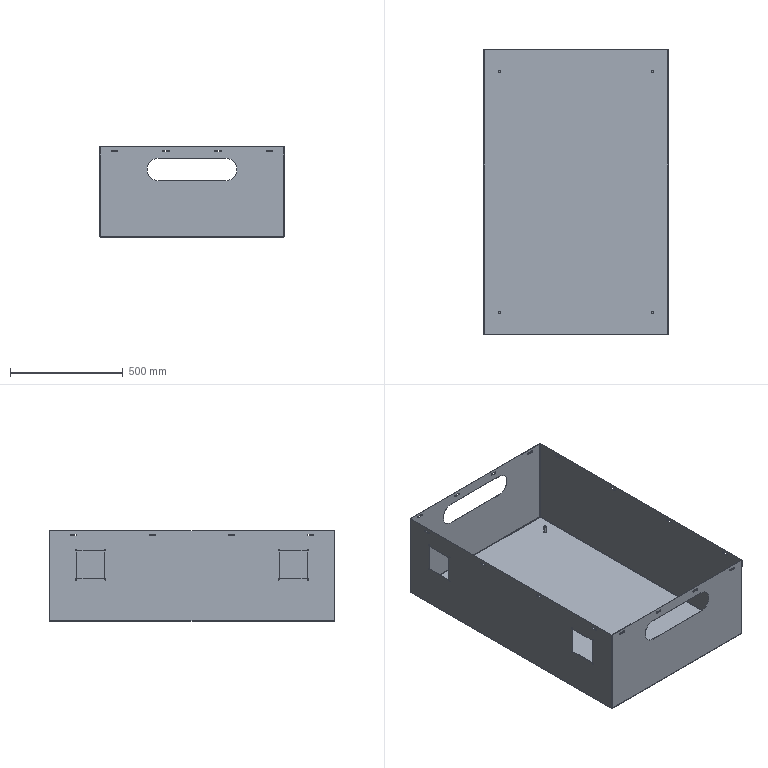Part | NX | features BREP 1 | 1 solid | 146 faces | box 820 x 1269 x 400 mm | volume 3889475 mm3 | plane 70 | cylinder 68 | spline 8 | commonest cylinder face diameters 8.2 x32 5 x16 10 x8 1.473 x4 4.473 x4 100 x4